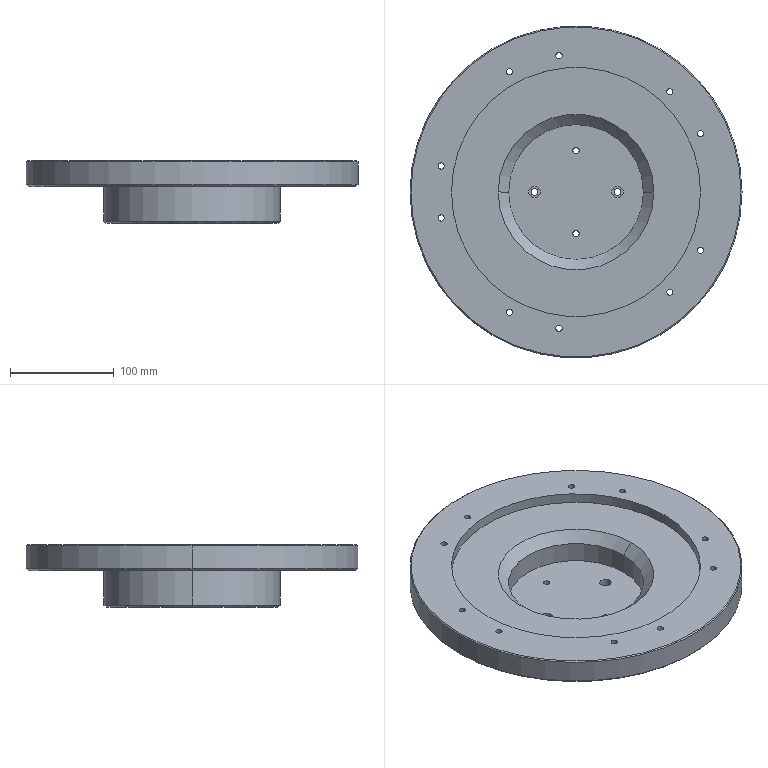NC program | NX | posted with a generic post | part box 320 x 320 x 60 mm
Lines 1 to 197 of 10816:
N10 G17 G21 G94 G90
(FLOOR_WALL , TOOL : D63)
N12 T01 M6
N14 G54
N16 G17 G0 G90 X-112.561 Y164.721 S6500 M3
N18 G43 Z90. H1
N20 Z66.
N22 G94 G1 Z63. F1250.
N24 X-107.151
N26 X107.155
N28 G2 X138.103 Y139.782 R195.661
N30 X138.335 Y139.552 R196.013
N32 X138.649 Y139.241 R195.738
N34 X143.474 Y134.27 R194.817
N36 G1 X-143.486
N38 G3 X-155.258 Y120.449 R194.528
N40 X-157.831 Y117.051 R193.916
N42 X-158.974 Y115.495 R195.834
N44 X-166.842 Y103.819 R194.954
N46 G1 X166.842
N48 G2 X182.294 Y73.368 R196.169
N50 G1 X-182.295
N52 G3 X-187.181 Y59.791 R195.834
N54 X-191.768 Y42.916 R195.006
N56 G1 X191.761
N58 G2 X195.377 Y21.038 R195.539
N60 X196.112 Y12.465 R194.105
N62 G1 X-196.109
N64 G3 X-196.19 Y11.115 R195.006
N66 X-196.5 Y1.125 R196.251
N68 G1 Y-1.105
N70 G3 X-195.683 Y-17.986 R194.105
N72 G1 X195.684
N74 G2 X190.446 Y-48.437 R195.007
N76 G1 X-190.439
N78 G3 X-189.757 Y-51.037 R195.539
N80 X-188.637 Y-55.026 R194.515
N82 G1 X-188.629 Y-55.054
N84 G3 X-184.517 Y-67.575 R195.249
N86 X-179.972 Y-78.888 R196.084
N88 G1 X179.977
N90 G2 X168.807 Y-100.592 R195.83
N92 X163.275 Y-109.339 R194.946
N94 G1 X-163.292
N96 G3 X-151.94 Y-124.61 R191.187
N98 X-144.931 Y-132.697 R194.815
N100 X-138.106 Y-139.79 R194.218
N102 G1 X138.111
N104 X142.349
N106 Z66.
N108 G0 Z90.
N110 X-112.561 Y164.721
N112 Z65.
N114 G1 Z62.
N116 X-107.151
N118 X107.155
N120 G2 X138.106 Y139.78 R195.661
N122 X138.333 Y139.554 R196.01
N124 X138.653 Y139.237 R195.738
N126 X143.474 Y134.27 R194.817
N128 G1 X-143.476
N130 G3 X-155.001 Y120.78 R193.916
N132 X-160.473 Y113.406 R195.719
N134 X-166.841 Y103.819 R195.834
N136 G1 X166.842
N138 G2 X182.294 Y73.368 R196.169
N140 G1 X-182.295
N142 G3 X-187.181 Y59.791 R195.834
N144 X-191.768 Y42.916 R195.006
N146 G1 X191.76
N148 G2 X194.22 Y29.843 R194.52
N150 X196.112 Y12.465 R194.105
N152 G1 X-196.109
N154 G3 X-196.241 Y10.147 R195.006
N156 X-196.5 Y0.898 R196.224
N158 G1 Y-1.069
N160 G3 X-195.683 Y-17.986 R194.105
N162 G1 X195.684
N164 G2 X190.446 Y-48.437 R195.007
N166 G1 X-190.439
N168 G3 X-189.726 Y-51.152 R194.519
N170 X-188.637 Y-55.026 R194.515
N172 X-184.496 Y-67.633 R195.245
N174 X-179.972 Y-78.888 R196.084
N176 G1 X179.977
N178 G2 X163.274 Y-109.339 R195.83
N180 G1 X-163.292
N182 G3 X-151.94 Y-124.61 R191.187
N184 X-144.932 Y-132.695 R194.815
N186 X-138.106 Y-139.79 R194.218
N188 G1 X138.101
N190 X142.338
N192 Z65.
N194 G0 Z90.
N196 X-112.56 Y164.722
N198 Z64.
N200 G1 Z61.
N202 X-107.15
N204 X107.154
N206 G2 X138.154 Y139.732 R195.661
N208 X138.327 Y139.56 R196.009
N210 X138.634 Y139.255 R196.075
N212 X143.473 Y134.271 R194.817
N214 G1 X-143.471
N216 G3 X-160.691 Y113.096 R195.686
N218 X-162.8 Y110.037 R195.719
N220 X-163.609 Y108.832 R195.525
N222 X-166.837 Y103.819 R195.594
N224 G1 X166.839
N226 G2 X169.635 Y99.187 R195.688
N228 X182.299 Y73.368 R195.874
N230 G1 X-182.292
N232 G3 X-182.928 Y71.767 R194.949
N234 X-191.773 Y42.917 R195.132
N236 G1 X191.76
N238 G2 X193.017 Y36.851 R194.52
N240 X195.735 Y17.348 R193.772
N242 X196.106 Y12.466 R196.058
N244 G1 X-196.108
N246 G3 X-196.37 Y7.223 R196.224
N248 X-196.5 Y1.462 R192.832
N250 G1 Y-1.466
N252 G3 X-196.33 Y-8.24 R192.832
N254 X-195.73 Y-17.397 R196.045
N256 X-195.678 Y-17.985 R193.783
N258 G1 X195.679
N260 G2 X195.51 Y-19.739 R196.226
N262 X190.453 Y-48.436 R195.137
N264 G1 X-190.439
N266 G3 X-190.078 Y-49.833 R194.519
N268 X-179.977 Y-78.888 R195.758
N270 G1 X179.971
N272 G2 X178.753 Y-81.607 R194.961
N274 X163.598 Y-108.849 R195.607
N276 X163.27 Y-109.339 R195.543
N278 G1 X-163.293
N280 G3 X-151.941 Y-124.609 R191.156
N282 X-144.995 Y-132.626 R194.815
N284 X-138.106 Y-139.79 R194.192
N286 G1 X138.101
N288 X142.338
N290 Z64.
N292 G0 Z90.
N294 X-112.56 Y164.722
N296 Z63.
N298 G1 Z60.
N300 X-107.15
N302 X107.154
N304 G2 X138.154 Y139.732 R195.661
N306 X138.327 Y139.56 R196.009
N308 X138.648 Y139.242 R196.075
N310 X143.473 Y134.271 R194.901
N312 G1 X-143.471
N314 G3 X-160.72 Y113.056 R195.686
N316 X-162.8 Y110.037 R195.719
N318 X-163.607 Y108.834 R195.524
N320 X-166.837 Y103.819 R195.594
N322 G1 X166.839
N324 G2 X169.163 Y99.989 R195.761
N326 X182.299 Y73.368 R195.874
N328 G1 X-182.292
N330 G3 X-182.929 Y71.765 R194.95
N332 X-191.773 Y42.917 R195.132
N334 G1 X191.76
N336 G2 X193.016 Y36.851 R194.519
N338 X195.735 Y17.35 R193.772
N340 X196.106 Y12.466 R196.057
N342 G1 X-196.108
N344 G3 X-196.37 Y7.223 R196.223
N346 X-196.5 Y1.462 R192.832
N348 G1 Y-1.466
N350 G3 X-196.33 Y-8.238 R192.832
N352 X-195.73 Y-17.398 R196.044
N354 X-195.678 Y-17.985 R193.783
N356 G1 X195.679
N358 G2 X195.51 Y-19.739 R196.226
N360 X190.453 Y-48.436 R195.137
N362 G1 X-190.439
N364 G3 X-190.078 Y-49.833 R194.519
N366 X-179.977 Y-78.888 R195.758
N368 G1 X179.971
N370 G2 X178.749 Y-81.616 R194.962
N372 X163.594 Y-108.854 R195.607
N374 X163.27 Y-109.339 R195.542
N376 G1 X-163.293
N378 G3 X-151.941 Y-124.609 R191.156
N380 X-144.995 Y-132.626 R194.815
N382 X-138.106 Y-139.79 R194.192
N384 G1 X138.101
N386 X142.338
N388 Z63.
N390 G0 Z90.
N392 M5